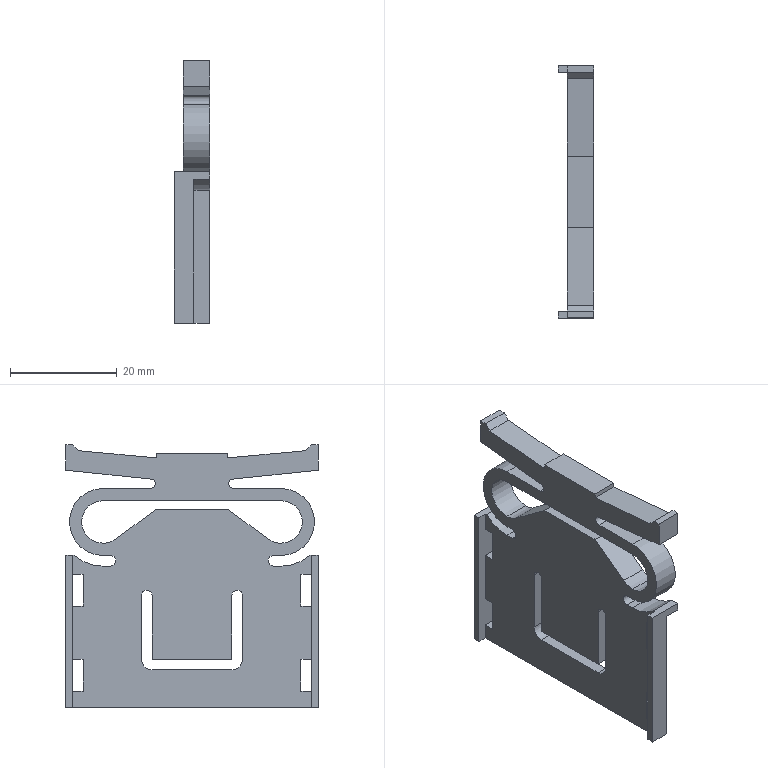Part | STEP file | K3HB_V_ADAPTER | 1 solid | 81 faces | box 6.7 x 47.4 x 49.3 mm | volume 5859 mm3 | plane 63 | cylinder 18 | commonest cylinder face diameters 2 x4 8 x4 1.739 x2 4 x2 12.6 x2 16.6 x2